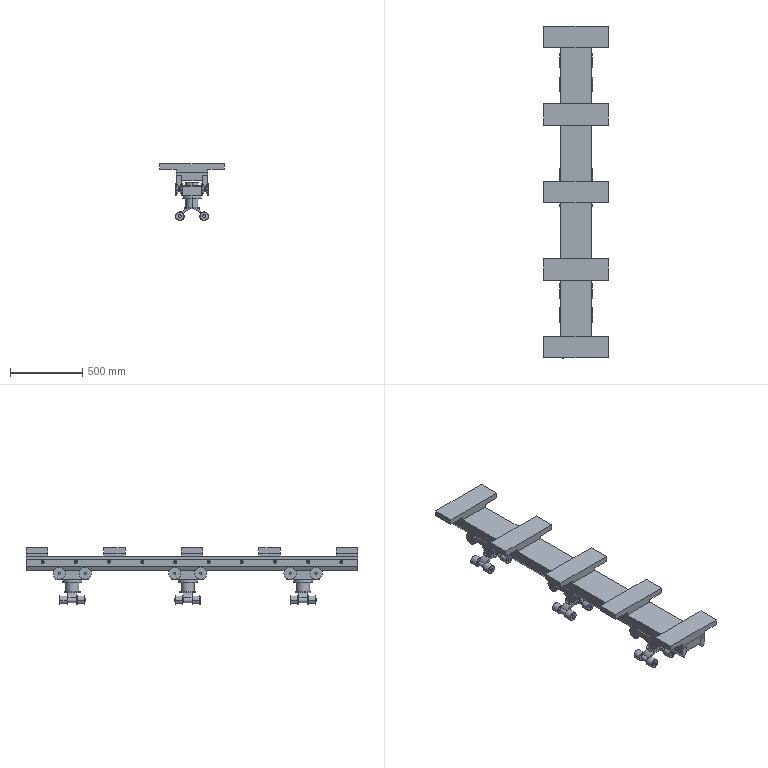Part | SolidWorks | features ReferencePattern 27, LocalLPattern 3, MirrorCompFeat 1 | 34 solids | 1077 faces | box 450 x 2300 x 395.088 mm | volume 64996675 mm3 | cylinder 467 | plane 434 | cone 176 | commonest cylinder face diameters 10 x80 20 x64 86 x48 8.5 x40 22 x40 16 x24